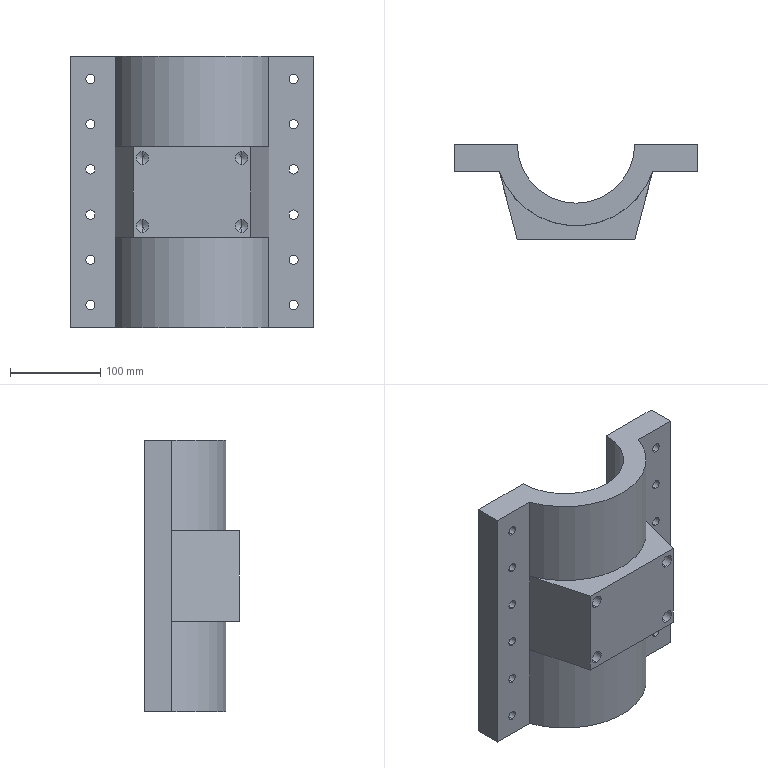Part | SolidWorks | features BaseBody 1 | 1 solid | 56 faces | box 270 x 105 x 300 mm | volume 2989960 mm3 | cylinder 35 | plane 13 | cone 8 | commonest cylinder face diameters 10.2 x24 14 x8 180 x2 130 x1